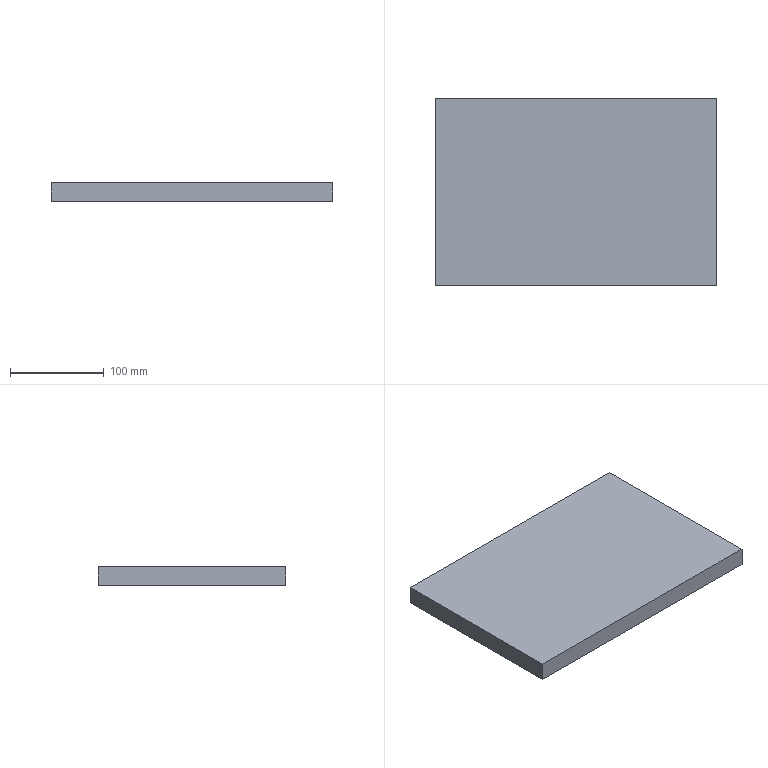Part | SolidWorks | features ICE 2, Extrusion 1 | 1 solid | 14 faces | box 300 x 200 x 20 mm | volume 751035 mm3 | plane 12 | cylinder 2 | commonest cylinder face diameters 60 x2
STEP:
#1=CARTESIAN_POINT('',(30.,0.,16.));
#2=VERTEX_POINT('',#1);
#3=CARTESIAN_POINT('',(-30.,0.,16.));
#4=VERTEX_POINT('',#3);
#5=CARTESIAN_POINT('',(0.,0.,16.));
#6=DIRECTION('',(0.,0.,-1.));
#7=DIRECTION('',(-1.,0.,0.));
#8=AXIS2_PLACEMENT_3D('',#5,#6,#7);
#9=CIRCLE('',#8,30.);
#10=EDGE_CURVE('',#2,#4,#9,.T.);
#11=ORIENTED_EDGE('',*,*,#10,.F.);
#12=CARTESIAN_POINT('',(30.,0.,10.));
#13=VERTEX_POINT('',#12);
#14=CARTESIAN_POINT('',(30.,0.,16.));
#15=DIRECTION('',(0.,0.,-1.));
#16=VECTOR('',#15,1000.);
#17=LINE('',#14,#16);
#18=EDGE_CURVE('',#2,#13,#17,.T.);
#19=ORIENTED_EDGE('',*,*,#18,.T.);
#20=CARTESIAN_POINT('',(-30.,0.,10.));
#21=VERTEX_POINT('',#20);
#22=CARTESIAN_POINT('',(0.,0.,10.));
#23=DIRECTION('',(0.,0.,-1.));
#24=DIRECTION('',(-1.,0.,0.));
#25=AXIS2_PLACEMENT_3D('',#22,#23,#24);
#26=CIRCLE('',#25,30.);
#27=EDGE_CURVE('',#13,#21,#26,.T.);
#28=ORIENTED_EDGE('',*,*,#27,.T.);
#29=CARTESIAN_POINT('',(-30.,0.,16.));
#30=DIRECTION('',(0.,0.,-1.));
#31=VECTOR('',#30,1000.);
#32=LINE('',#29,#31);
#33=EDGE_CURVE('',#4,#21,#32,.T.);
#34=ORIENTED_EDGE('',*,*,#33,.F.);
#35=EDGE_LOOP('',(#11,#19,#28,#34));
#36=FACE_OUTER_BOUND('',#35,.T.);
#37=CARTESIAN_POINT('',(0.,0.,16.));
#38=DIRECTION('',(0.,0.,-1.));
#39=DIRECTION('',(-1.,0.,0.));
#40=AXIS2_PLACEMENT_3D('',#37,#38,#39);
#41=CYLINDRICAL_SURFACE('',#40,30.);
#42=ADVANCED_FACE('',(#36),#41,.F.);
#43=CARTESIAN_POINT('',(150.,-100.,0.));
#44=VERTEX_POINT('',#43);
#45=CARTESIAN_POINT('',(150.,100.,0.));
#46=VERTEX_POINT('',#45);
#47=CARTESIAN_POINT('',(150.,100.,0.));
#48=DIRECTION('',(0.,1.,0.));
#49=VECTOR('',#48,1000.);
#50=LINE('',#47,#49);
#51=EDGE_CURVE('',#44,#46,#50,.T.);
#52=ORIENTED_EDGE('',*,*,#51,.T.);
#53=CARTESIAN_POINT('',(150.,100.,20.));
#54=VERTEX_POINT('',#53);
#55=CARTESIAN_POINT('',(150.,100.,20.));
#56=DIRECTION('',(0.,0.,-1.));
#57=VECTOR('',#56,1000.);
#58=LINE('',#55,#57);
#59=EDGE_CURVE('',#54,#46,#58,.T.);
#60=ORIENTED_EDGE('',*,*,#59,.F.);
#61=CARTESIAN_POINT('',(150.,-100.,20.));
#62=VERTEX_POINT('',#61);
#63=CARTESIAN_POINT('',(150.,100.,20.));
#64=DIRECTION('',(0.,1.,0.));
#65=VECTOR('',#64,1000.);
#66=LINE('',#63,#65);
#67=EDGE_CURVE('',#62,#54,#66,.T.);
#68=ORIENTED_EDGE('',*,*,#67,.F.);
#69=CARTESIAN_POINT('',(150.,-100.,20.));
#70=DIRECTION('',(0.,0.,-1.));
#71=VECTOR('',#70,1000.);
#72=LINE('',#69,#71);
#73=EDGE_CURVE('',#62,#44,#72,.T.);
#74=ORIENTED_EDGE('',*,*,#73,.T.);
#75=EDGE_LOOP('',(#52,#60,#68,#74));
#76=FACE_OUTER_BOUND('',#75,.T.);
#77=CARTESIAN_POINT('',(150.,100.,20.));
#78=DIRECTION('',(-1.,0.,0.));
#79=DIRECTION('',(0.,0.,1.));
#80=AXIS2_PLACEMENT_3D('',#77,#78,#79);
#81=PLANE('',#80);
#82=ADVANCED_FACE('',(#76),#81,.F.);
#83=CARTESIAN_POINT('',(-150.,100.,0.));
#84=VERTEX_POINT('',#83);
#85=CARTESIAN_POINT('',(-150.,100.,0.));
#86=DIRECTION('',(-1.,0.,0.));
#87=VECTOR('',#86,1000.);
#88=LINE('',#85,#87);
#89=EDGE_CURVE('',#46,#84,#88,.T.);
#90=ORIENTED_EDGE('',*,*,#89,.T.);
#91=CARTESIAN_POINT('',(-150.,100.,20.));
#92=VERTEX_POINT('',#91);
#93=CARTESIAN_POINT('',(-150.,100.,20.));
#94=DIRECTION('',(0.,0.,-1.));
#95=VECTOR('',#94,1000.);
#96=LINE('',#93,#95);
#97=EDGE_CURVE('',#92,#84,#96,.T.);
#98=ORIENTED_EDGE('',*,*,#97,.F.);
#99=CARTESIAN_POINT('',(-150.,100.,20.));
#100=DIRECTION('',(-1.,0.,0.));
#101=VECTOR('',#100,1000.);
#102=LINE('',#99,#101);
#103=EDGE_CURVE('',#54,#92,#102,.T.);
#104=ORIENTED_EDGE('',*,*,#103,.F.);
#105=ORIENTED_EDGE('',*,*,#59,.T.);
#106=EDGE_LOOP('',(#90,#98,#104,#105));
#107=FACE_OUTER_BOUND('',#106,.T.);
#108=CARTESIAN_POINT('',(-150.,100.,20.));
#109=DIRECTION('',(0.,-1.,0.));
#110=DIRECTION('',(0.,0.,-1.));
#111=AXIS2_PLACEMENT_3D('',#108,#109,#110);
#112=PLANE('',#111);
#113=ADVANCED_FACE('',(#107),#112,.F.);
#114=CARTESIAN_POINT('',(-150.,-100.,0.));
#115=VERTEX_POINT('',#114);
#116=CARTESIAN_POINT('',(-150.,100.,0.));
#117=DIRECTION('',(0.,-1.,0.));
#118=VECTOR('',#117,1000.);
#119=LINE('',#116,#118);
#120=EDGE_CURVE('',#84,#115,#119,.T.);
#121=ORIENTED_EDGE('',*,*,#120,.T.);
#122=CARTESIAN_POINT('',(-150.,-100.,20.));
#123=VERTEX_POINT('',#122);
#124=CARTESIAN_POINT('',(-150.,-100.,20.));
#125=DIRECTION('',(0.,0.,-1.));
#126=VECTOR('',#125,1000.);
#127=LINE('',#124,#126);
#128=EDGE_CURVE('',#123,#115,#127,.T.);
#129=ORIENTED_EDGE('',*,*,#128,.F.);
#130=CARTESIAN_POINT('',(-150.,100.,20.));
#131=DIRECTION('',(0.,-1.,0.));
#132=VECTOR('',#131,1000.);
#133=LINE('',#130,#132);
#134=EDGE_CURVE('',#92,#123,#133,.T.);
#135=ORIENTED_EDGE('',*,*,#134,.F.);
#136=ORIENTED_EDGE('',*,*,#97,.T.);
#137=EDGE_LOOP('',(#121,#129,#135,#136));
#138=FACE_OUTER_BOUND('',#137,.T.);
#139=CARTESIAN_POINT('',(-150.,100.,20.));
#140=DIRECTION('',(1.,0.,0.));
#141=DIRECTION('',(0.,0.,-1.));
#142=AXIS2_PLACEMENT_3D('',#139,#140,#141);
#143=PLANE('',#142);
#144=ADVANCED_FACE('',(#138),#143,.F.);
#145=CARTESIAN_POINT('',(-150.,-100.,0.));
#146=DIRECTION('',(1.,0.,0.));
#147=VECTOR('',#146,1000.);
#148=LINE('',#145,#147);
#149=EDGE_CURVE('',#115,#44,#148,.T.);
#150=ORIENTED_EDGE('',*,*,#149,.T.);
#151=ORIENTED_EDGE('',*,*,#73,.F.);
#152=CARTESIAN_POINT('',(-150.,-100.,20.));
#153=DIRECTION('',(1.,0.,0.));
#154=VECTOR('',#153,1000.);
#155=LINE('',#152,#154);
#156=EDGE_CURVE('',#123,#62,#155,.T.);
#157=ORIENTED_EDGE('',*,*,#156,.F.);
#158=ORIENTED_EDGE('',*,*,#128,.T.);
#159=EDGE_LOOP('',(#150,#151,#157,#158));
#160=FACE_OUTER_BOUND('',#159,.T.);
#161=CARTESIAN_POINT('',(-150.,-100.,20.));
#162=DIRECTION('',(0.,1.,0.));
#163=DIRECTION('',(0.,0.,1.));
#164=AXIS2_PLACEMENT_3D('',#161,#162,#163);
#165=PLANE('',#164);
#166=ADVANCED_FACE('',(#160),#165,.F.);
#167=ORIENTED_EDGE('',*,*,#67,.T.);
#168=ORIENTED_EDGE('',*,*,#103,.T.);
#169=ORIENTED_EDGE('',*,*,#134,.T.);
#170=ORIENTED_EDGE('',*,*,#156,.T.);
#171=EDGE_LOOP('',(#167,#168,#169,#170));
#172=FACE_OUTER_BOUND('',#171,.T.);
#173=CARTESIAN_POINT('',(0.,0.,20.));
#174=DIRECTION('',(0.,0.,1.));
#175=DIRECTION('',(1.,0.,0.));
#176=AXIS2_PLACEMENT_3D('',#173,#174,#175);
#177=PLANE('',#176);
#178=ADVANCED_FACE('',(#172),#177,.T.);
#179=CARTESIAN_POINT('',(-135.,80.,0.));
#180=VERTEX_POINT('',#179);
#181=CARTESIAN_POINT('',(135.,80.,0.));
#182=VERTEX_POINT('',#181);
#183=CARTESIAN_POINT('',(135.,80.,0.));
#184=DIRECTION('',(1.,0.,0.));
#185=VECTOR('',#184,1000.);
#186=LINE('',#183,#185);
#187=EDGE_CURVE('',#180,#182,#186,.T.);
#188=ORIENTED_EDGE('',*,*,#187,.F.);
#189=CARTESIAN_POINT('',(-135.,-80.,0.));
#190=VERTEX_POINT('',#189);
#191=CARTESIAN_POINT('',(-135.,80.,0.));
#192=DIRECTION('',(0.,1.,0.));
#193=VECTOR('',#192,1000.);
#194=LINE('',#191,#193);
#195=EDGE_CURVE('',#190,#180,#194,.T.);
#196=ORIENTED_EDGE('',*,*,#195,.F.);
#197=CARTESIAN_POINT('',(135.,-80.,0.));
#198=VERTEX_POINT('',#197);
#199=CARTESIAN_POINT('',(135.,-80.,0.));
#200=DIRECTION('',(-1.,0.,0.));
#201=VECTOR('',#200,1000.);
#202=LINE('',#199,#201);
#203=EDGE_CURVE('',#198,#190,#202,.T.);
#204=ORIENTED_EDGE('',*,*,#203,.F.);
#205=CARTESIAN_POINT('',(135.,80.,0.));
#206=DIRECTION('',(0.,-1.,0.));
#207=VECTOR('',#206,1000.);
#208=LINE('',#205,#207);
#209=EDGE_CURVE('',#182,#198,#208,.T.);
#210=ORIENTED_EDGE('',*,*,#209,.F.);
#211=EDGE_LOOP('',(#188,#196,#204,#210));
#212=FACE_BOUND('',#211,.T.);
#213=ORIENTED_EDGE('',*,*,#51,.F.);
#214=ORIENTED_EDGE('',*,*,#149,.F.);
#215=ORIENTED_EDGE('',*,*,#120,.F.);
#216=ORIENTED_EDGE('',*,*,#89,.F.);
#217=EDGE_LOOP('',(#213,#214,#215,#216));
#218=FACE_OUTER_BOUND('',#217,.T.);
#219=CARTESIAN_POINT('',(0.,0.,0.));
#220=DIRECTION('',(0.,0.,1.));
#221=DIRECTION('',(1.,0.,0.));
#222=AXIS2_PLACEMENT_3D('',#219,#220,#221);
#223=PLANE('',#222);
#224=ADVANCED_FACE('',(#212,#218),#223,.F.);
#225=ORIENTED_EDGE('',*,*,#195,.T.);
#226=CARTESIAN_POINT('',(-135.,80.,10.));
#227=VERTEX_POINT('',#226);
#228=CARTESIAN_POINT('',(-135.,80.,10.));
#229=DIRECTION('',(0.,0.,-1.));
#230=VECTOR('',#229,1000.);
#231=LINE('',#228,#230);
#232=EDGE_CURVE('',#227,#180,#231,.T.);
#233=ORIENTED_EDGE('',*,*,#232,.F.);
#234=CARTESIAN_POINT('',(-135.,-80.,10.));
#235=VERTEX_POINT('',#234);
#236=CARTESIAN_POINT('',(-135.,80.,10.));
#237=DIRECTION('',(0.,1.,0.));
#238=VECTOR('',#237,1000.);
#239=LINE('',#236,#238);
#240=EDGE_CURVE('',#235,#227,#239,.T.);
#241=ORIENTED_EDGE('',*,*,#240,.F.);
#242=CARTESIAN_POINT('',(-135.,-80.,10.));
#243=DIRECTION('',(0.,0.,-1.));
#244=VECTOR('',#243,1000.);
#245=LINE('',#242,#244);
#246=EDGE_CURVE('',#235,#190,#245,.T.);
#247=ORIENTED_EDGE('',*,*,#246,.T.);
#248=EDGE_LOOP('',(#225,#233,#241,#247));
#249=FACE_OUTER_BOUND('',#248,.T.);
#250=CARTESIAN_POINT('',(-135.,80.,10.));
#251=DIRECTION('',(-1.,0.,0.));
#252=DIRECTION('',(0.,0.,1.));
#253=AXIS2_PLACEMENT_3D('',#250,#251,#252);
#254=PLANE('',#253);
#255=ADVANCED_FACE('',(#249),#254,.F.);
#256=ORIENTED_EDGE('',*,*,#203,.T.);
#257=ORIENTED_EDGE('',*,*,#246,.F.);
#258=CARTESIAN_POINT('',(135.,-80.,10.));
#259=VERTEX_POINT('',#258);
#260=CARTESIAN_POINT('',(135.,-80.,10.));
#261=DIRECTION('',(-1.,0.,0.));
#262=VECTOR('',#261,1000.);
#263=LINE('',#260,#262);
#264=EDGE_CURVE('',#259,#235,#263,.T.);
#265=ORIENTED_EDGE('',*,*,#264,.F.);
#266=CARTESIAN_POINT('',(135.,-80.,10.));
#267=DIRECTION('',(0.,0.,-1.));
#268=VECTOR('',#267,1000.);
#269=LINE('',#266,#268);
#270=EDGE_CURVE('',#259,#198,#269,.T.);
#271=ORIENTED_EDGE('',*,*,#270,.T.);
#272=EDGE_LOOP('',(#256,#257,#265,#271));
#273=FACE_OUTER_BOUND('',#272,.T.);
#274=CARTESIAN_POINT('',(135.,-80.,10.));
#275=DIRECTION('',(0.,-1.,0.));
#276=DIRECTION('',(0.,0.,-1.));
#277=AXIS2_PLACEMENT_3D('',#274,#275,#276);
#278=PLANE('',#277);
#279=ADVANCED_FACE('',(#273),#278,.F.);
#280=ORIENTED_EDGE('',*,*,#209,.T.);
#281=ORIENTED_EDGE('',*,*,#270,.F.);
#282=CARTESIAN_POINT('',(135.,80.,10.));
#283=VERTEX_POINT('',#282);
#284=CARTESIAN_POINT('',(135.,80.,10.));
#285=DIRECTION('',(0.,-1.,0.));
#286=VECTOR('',#285,1000.);
#287=LINE('',#284,#286);
#288=EDGE_CURVE('',#283,#259,#287,.T.);
#289=ORIENTED_EDGE('',*,*,#288,.F.);
#290=CARTESIAN_POINT('',(135.,80.,10.));
#291=DIRECTION('',(0.,0.,-1.));
#292=VECTOR('',#291,1000.);
#293=LINE('',#290,#292);
#294=EDGE_CURVE('',#283,#182,#293,.T.);
#295=ORIENTED_EDGE('',*,*,#294,.T.);
#296=EDGE_LOOP('',(#280,#281,#289,#295));
#297=FACE_OUTER_BOUND('',#296,.T.);
#298=CARTESIAN_POINT('',(135.,80.,10.));
#299=DIRECTION('',(1.,0.,0.));
#300=DIRECTION('',(0.,0.,-1.));
#301=AXIS2_PLACEMENT_3D('',#298,#299,#300);
#302=PLANE('',#301);
#303=ADVANCED_FACE('',(#297),#302,.F.);
#304=ORIENTED_EDGE('',*,*,#187,.T.);
#305=ORIENTED_EDGE('',*,*,#294,.F.);
#306=CARTESIAN_POINT('',(135.,80.,10.));
#307=DIRECTION('',(1.,0.,0.));
#308=VECTOR('',#307,1000.);
#309=LINE('',#306,#308);
#310=EDGE_CURVE('',#227,#283,#309,.T.);
#311=ORIENTED_EDGE('',*,*,#310,.F.);
#312=ORIENTED_EDGE('',*,*,#232,.T.);
#313=EDGE_LOOP('',(#304,#305,#311,#312));
#314=FACE_OUTER_BOUND('',#313,.T.);
#315=CARTESIAN_POINT('',(135.,80.,10.));
#316=DIRECTION('',(0.,1.,0.));
#317=DIRECTION('',(0.,0.,1.));
#318=AXIS2_PLACEMENT_3D('',#315,#316,#317);
#319=PLANE('',#318);
#320=ADVANCED_FACE('',(#314),#319,.F.);
#321=CARTESIAN_POINT('',(0.,0.,10.));
#322=DIRECTION('',(0.,0.,-1.));
#323=DIRECTION('',(-1.,0.,0.));
#324=AXIS2_PLACEMENT_3D('',#321,#322,#323);
#325=CIRCLE('',#324,30.);
#326=EDGE_CURVE('',#21,#13,#325,.T.);
#327=ORIENTED_EDGE('',*,*,#326,.F.);
#328=ORIENTED_EDGE('',*,*,#27,.F.);
#329=EDGE_LOOP('',(#327,#328));
#330=FACE_BOUND('',#329,.T.);
#331=ORIENTED_EDGE('',*,*,#240,.T.);
#332=ORIENTED_EDGE('',*,*,#310,.T.);
#333=ORIENTED_EDGE('',*,*,#288,.T.);
#334=ORIENTED_EDGE('',*,*,#264,.T.);
#335=EDGE_LOOP('',(#331,#332,#333,#334));
#336=FACE_OUTER_BOUND('',#335,.T.);
#337=CARTESIAN_POINT('',(0.,0.,10.));
#338=DIRECTION('',(0.,0.,-1.));
#339=DIRECTION('',(-1.,0.,0.));
#340=AXIS2_PLACEMENT_3D('',#337,#338,#339);
#341=PLANE('',#340);
#342=ADVANCED_FACE('',(#330,#336),#341,.T.);
#343=ORIENTED_EDGE('',*,*,#18,.F.);
#344=CARTESIAN_POINT('',(0.,0.,16.));
#345=DIRECTION('',(0.,0.,-1.));
#346=DIRECTION('',(-1.,0.,0.));
#347=AXIS2_PLACEMENT_3D('',#344,#345,#346);
#348=CIRCLE('',#347,30.);
#349=EDGE_CURVE('',#4,#2,#348,.T.);
#350=ORIENTED_EDGE('',*,*,#349,.F.);
#351=ORIENTED_EDGE('',*,*,#33,.T.);
#352=ORIENTED_EDGE('',*,*,#326,.T.);
#353=EDGE_LOOP('',(#343,#350,#351,#352));
#354=FACE_OUTER_BOUND('',#353,.T.);
#355=CARTESIAN_POINT('',(0.,0.,16.));
#356=DIRECTION('',(0.,0.,-1.));
#357=DIRECTION('',(-1.,0.,0.));
#358=AXIS2_PLACEMENT_3D('',#355,#356,#357);
#359=CYLINDRICAL_SURFACE('',#358,30.);
#360=ADVANCED_FACE('',(#354),#359,.F.);
#361=ORIENTED_EDGE('',*,*,#349,.T.);
#362=ORIENTED_EDGE('',*,*,#10,.T.);
#363=EDGE_LOOP('',(#361,#362));
#364=FACE_OUTER_BOUND('',#363,.T.);
#365=CARTESIAN_POINT('',(0.,0.,16.));
#366=DIRECTION('',(0.,0.,-1.));
#367=DIRECTION('',(-1.,0.,0.));
#368=AXIS2_PLACEMENT_3D('',#365,#366,#367);
#369=PLANE('',#368);
#370=ADVANCED_FACE('',(#364),#369,.T.);
#371=CLOSED_SHELL('',(#42,#82,#113,#144,#166,#178,#224,#255,#279,#303,#320,#342,#360,#370));
#372=MANIFOLD_SOLID_BREP('',#371);
#373=CARTESIAN_POINT('',(0.,0.,0.));
#374=DIRECTION('',(0.,0.,1.));
#375=DIRECTION('',(1.,0.,0.));
#376=AXIS2_PLACEMENT_3D('',#373,#374,#375);
#377=(LENGTH_UNIT()NAMED_UNIT(*)SI_UNIT(.MILLI.,.METRE.));
#378=UNCERTAINTY_MEASURE_WITH_UNIT(LENGTH_MEASURE(0.00001),#377,'','');
#379=(NAMED_UNIT(*)PLANE_ANGLE_UNIT()SI_UNIT($,.RADIAN.));
#380=(NAMED_UNIT(*)SI_UNIT($,.STERADIAN.)SOLID_ANGLE_UNIT());
#381=(GEOMETRIC_REPRESENTATION_CONTEXT(3)GLOBAL_UNCERTAINTY_ASSIGNED_CONTEXT((#378))GLOBAL_UNIT_ASSIGNED_CONTEXT((#377,#379,#380))REPRESENTATION_CONTEXT('',''));
#382=ADVANCED_BREP_SHAPE_REPRESENTATION('',(#372,#376),#381);